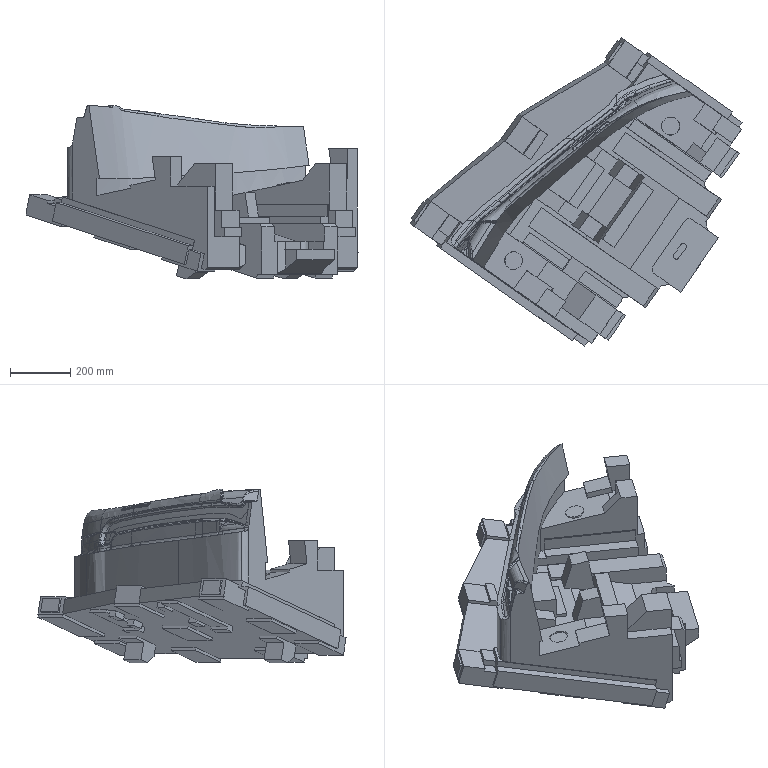Part | NX | features solid 2 | 1 solid | 518 faces | box 1105 x 1026 x 578.555 mm | volume 94031473 mm3 | plane 271 | spline 241 | cylinder 6 | commonest cylinder face diameters 20 x2 40 x2 60 x2